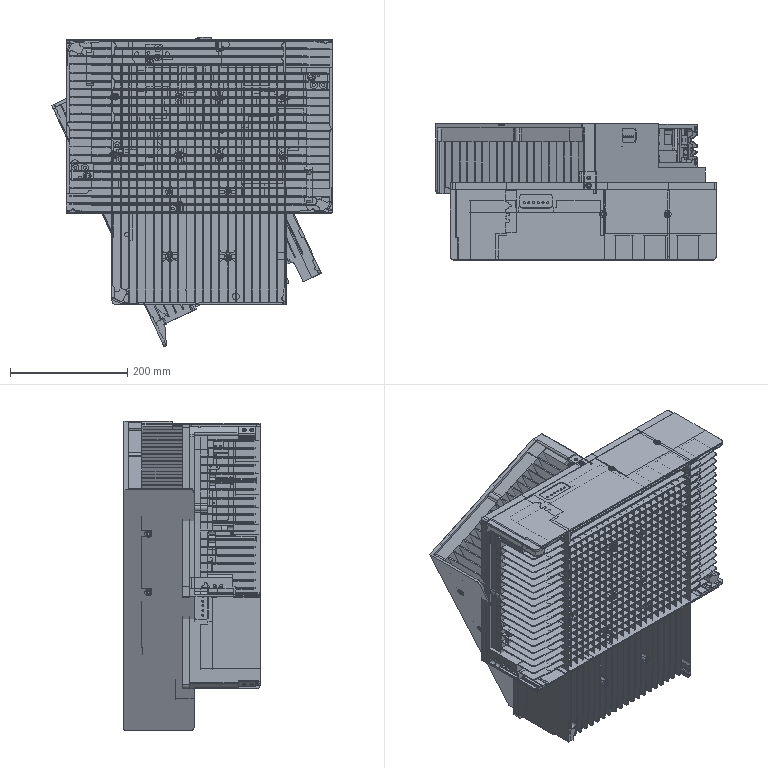NC program | NX | posted with a generic post
Whole program:
N10 G17 G21 G94 G90
(HOLE_MILLING_4 , TOOL : D4_J)
N12 T05 M6
N14 G53
N16 G17 G0 G90 X9.346 Y7. S2500 M3
N18 G43 Z20. H5
N20 Z0.1
N22 G94 G3 X9.846 Y6.5 R0.5 F1000.
N24 X10.346 Y7. R0.5
N26 X10.346 Y7. Z0.05 I-1. J0.
N28 X10.346 Y7. Z0. I-1. J0.
N30 X10.346 Y7. Z-0.05 I-1. J0.
N32 X10.346 Y7. Z-0.1 I-1. J0.
N34 X10.346 Y7. Z-0.15 I-1. J0.
N36 X10.346 Y7. Z-0.2 I-1. J0.
N38 X10.346 Y7. Z-0.25 I-1. J0.
N40 X10.346 Y7. Z-0.3 I-1. J0.
N42 X10.346 Y7. Z-0.35 I-1. J0.
N44 X10.346 Y7. Z-0.4 I-1. J0.
N46 X10.346 Y7. Z-0.45 I-1. J0.
N48 X10.346 Y7. Z-0.5 I-1. J0.
N50 X10.346 Y7. Z-0.55 I-1. J0.
N52 X10.346 Y7. Z-0.6 I-1. J0.
N54 X10.346 Y7. Z-0.65 I-1. J0.
N56 X10.346 Y7. Z-0.7 I-1. J0.
N58 X10.346 Y7. Z-0.75 I-1. J0.
N60 X10.346 Y7. Z-0.8 I-1. J0.
N62 X10.346 Y7. Z-0.85 I-1. J0.
N64 X10.346 Y7. Z-0.9 I-1. J0.
N66 X10.346 Y7. Z-0.95 I-1. J0.
N68 X10.346 Y7. Z-1. I-1. J0.
N70 X10.346 Y7. Z-1.05 I-1. J0.
N72 X10.346 Y7. Z-1.1 I-1. J0.
N74 X10.346 Y7. Z-1.15 I-1. J0.
N76 X10.346 Y7. Z-1.2 I-1. J0.
N78 X10.346 Y7. Z-1.25 I-1. J0.
N80 X10.346 Y7. Z-1.3 I-1. J0.
N82 X10.346 Y7. Z-1.35 I-1. J0.
N84 X10.346 Y7. Z-1.4 I-1. J0.
N86 X10.346 Y7. Z-1.45 I-1. J0.
N88 X10.346 Y7. Z-1.5 I-1. J0.
N90 X10.346 Y7. Z-1.55 I-1. J0.
N92 X10.346 Y7. Z-1.6 I-1. J0.
N94 X10.346 Y7. Z-1.65 I-1. J0.
N96 X10.346 Y7. Z-1.7 I-1. J0.
N98 X10.346 Y7. Z-1.75 I-1. J0.
N100 X10.346 Y7. Z-1.8 I-1. J0.
N102 X10.346 Y7. Z-1.85 I-1. J0.
N104 X10.346 Y7. Z-1.9 I-1. J0.
N106 X10.346 Y7. Z-1.95 I-1. J0.
N108 X10.346 Y7. Z-2. I-1. J0.
N110 X10.346 Y7. Z-2.05 I-1. J0.
N112 X10.346 Y7. Z-2.1 I-1. J0.
N114 X10.346 Y7. Z-2.15 I-1. J0.
N116 X10.346 Y7. Z-2.2 I-1. J0.
N118 X10.346 Y7. Z-2.25 I-1. J0.
N120 X10.346 Y7. Z-2.3 I-1. J0.
N122 X10.346 Y7. Z-2.35 I-1. J0.
N124 X10.346 Y7. Z-2.4 I-1. J0.
N126 X10.346 Y7. Z-2.45 I-1. J0.
N128 X10.346 Y7. Z-2.5 I-1. J0.
N130 X10.346 Y7. Z-2.55 I-1. J0.
N132 X10.346 Y7. Z-2.6 I-1. J0.
N134 X10.346 Y7. Z-2.65 I-1. J0.
N136 X10.346 Y7. Z-2.7 I-1. J0.
N138 X10.346 Y7. Z-2.75 I-1. J0.
N140 X10.346 Y7. Z-2.8 I-1. J0.
N142 X10.346 Y7. Z-2.85 I-1. J0.
N144 X10.346 Y7. Z-2.9 I-1. J0.
N146 X10.346 Y7. Z-2.95 I-1. J0.
N148 X10.346 Y7. Z-3. I-1. J0.
N150 X10.346 Y7. Z-3.05 I-1. J0.
N152 X10.346 Y7. Z-3.1 I-1. J0.
N154 X10.346 Y7. Z-3.15 I-1. J0.
N156 X10.346 Y7. Z-3.2 I-1. J0.
N158 X10.346 Y7. Z-3.25 I-1. J0.
N160 X10.346 Y7. Z-3.3 I-1. J0.
N162 X10.346 Y7. Z-3.35 I-1. J0.
N164 X10.346 Y7. Z-3.4 I-1. J0.
N166 X10.346 Y7. Z-3.45 I-1. J0.
N168 X10.346 Y7. Z-3.5 I-1. J0.
N170 X10.346 Y7. Z-3.55 I-1. J0.
N172 X10.346 Y7. Z-3.6 I-1. J0.
N174 X10.346 Y7. Z-3.65 I-1. J0.
N176 X10.346 Y7. Z-3.7 I-1. J0.
N178 X10.346 Y7. Z-3.75 I-1. J0.
N180 X10.346 Y7. Z-3.8 I-1. J0.
N182 X10.346 Y7. Z-3.85 I-1. J0.
N184 X10.346 Y7. Z-3.9 I-1. J0.
N186 X10.346 Y7. Z-3.95 I-1. J0.
N188 X10.346 Y7. Z-4. I-1. J0.
N190 X10.346 Y7. Z-4.05 I-1. J0.
N192 X10.346 Y7. Z-4.1 I-1. J0.
N194 X10.346 Y7. Z-4.15 I-1. J0.
N196 X10.346 Y7. Z-4.2 I-1. J0.
N198 X10.346 Y7. Z-4.25 I-1. J0.
N200 X10.346 Y7. Z-4.3 I-1. J0.
N202 X10.346 Y7. Z-4.35 I-1. J0.
N204 X10.346 Y7. Z-4.4 I-1. J0.
N206 X10.346 Y7. Z-4.45 I-1. J0.
N208 X10.346 Y7. Z-4.5 I-1. J0.
N210 X10.346 Y7. Z-4.55 I-1. J0.
N212 X10.346 Y7. Z-4.6 I-1. J0.
N214 X10.346 Y7. Z-4.65 I-1. J0.
N216 X10.346 Y7. Z-4.7 I-1. J0.
N218 X10.346 Y7. Z-4.75 I-1. J0.
N220 X10.346 Y7. Z-4.8 I-1. J0.
N222 X10.346 Y7. Z-4.85 I-1. J0.
N224 X10.346 Y7. Z-4.9 I-1. J0.
N226 X10.346 Y7. Z-4.95 I-1. J0.
N228 X10.346 Y7. Z-5. I-1. J0.
N230 X10.346 Y7. Z-5.05 I-1. J0.
N232 X10.346 Y7. Z-5.1 I-1. J0.
N234 X10.346 Y7. Z-5.15 I-1. J0.
N236 X10.346 Y7. Z-5.2 I-1. J0.
N238 X10.346 Y7. Z-5.25 I-1. J0.
N240 X10.346 Y7. Z-5.3 I-1. J0.
N242 X10.346 Y7. Z-5.35 I-1. J0.
N244 X10.346 Y7. Z-5.4 I-1. J0.
N246 X10.346 Y7. Z-5.45 I-1. J0.
N248 X10.346 Y7. Z-5.5 I-1. J0.
N250 X10.346 Y7. Z-5.55 I-1. J0.
N252 X10.346 Y7. Z-5.6 I-1. J0.
N254 X10.346 Y7. Z-5.65 I-1. J0.
N256 X10.346 Y7. Z-5.7 I-1. J0.
N258 X10.346 Y7. Z-5.75 I-1. J0.
N260 X10.346 Y7. Z-5.8 I-1. J0.
N262 X10.346 Y7. Z-5.85 I-1. J0.
N264 X10.346 Y7. Z-5.9 I-1. J0.
N266 X10.346 Y7. Z-5.95 I-1. J0.
N268 X10.346 Y7. Z-6. I-1. J0.
N270 X10.346 Y7. Z-6.05 I-1. J0.
N272 X10.346 Y7. Z-6.1 I-1. J0.
N274 X10.346 Y7. Z-6.15 I-1. J0.
N276 X10.346 Y7. Z-6.2 I-1. J0.
N278 X10.346 Y7. Z-6.25 I-1. J0.
N280 X10.346 Y7. Z-6.3 I-1. J0.
N282 X10.346 Y7. Z-6.35 I-1. J0.
N284 X10.346 Y7. Z-6.4 I-1. J0.
N286 X10.346 Y7. Z-6.45 I-1. J0.
N288 X10.346 Y7. Z-6.5 I-1. J0.
N290 X10.346 Y7. Z-6.55 I-1. J0.
N292 X10.346 Y7. Z-6.6 I-1. J0.
N294 X10.346 Y7. Z-6.65 I-1. J0.
N296 X10.346 Y7. Z-6.7 I-1. J0.
N298 X10.346 Y7. Z-6.75 I-1. J0.
N300 X10.346 Y7. Z-6.8 I-1. J0.
N302 X10.346 Y7. Z-6.85 I-1. J0.
N304 X10.346 Y7. Z-6.9 I-1. J0.
N306 X10.346 Y7. Z-6.95 I-1. J0.
N308 X10.346 Y7. Z-7. I-1. J0.
N310 X10.346 Y7. Z-7.05 I-1. J0.
N312 X10.346 Y7. Z-7.1 I-1. J0.
N314 X10.346 Y7. Z-7.15 I-1. J0.
N316 X10.346 Y7. Z-7.2 I-1. J0.
N318 X10.346 Y7. Z-7.25 I-1. J0.
N320 X10.346 Y7. Z-7.3 I-1. J0.
N322 X10.346 Y7. Z-7.35 I-1. J0.
N324 X10.346 Y7. Z-7.4 I-1. J0.
N326 X10.346 Y7. Z-7.45 I-1. J0.
N328 X10.346 Y7. Z-7.5 I-1. J0.
N330 X10.346 Y7. Z-7.55 I-1. J0.
N332 X10.346 Y7. Z-7.6 I-1. J0.
N334 X10.346 Y7. Z-7.65 I-1. J0.
N336 X10.346 Y7. Z-7.7 I-1. J0.
N338 X10.346 Y7. Z-7.75 I-1. J0.
N340 X10.346 Y7. Z-7.8 I-1. J0.
N342 X10.346 Y7. Z-7.85 I-1. J0.
N344 X10.346 Y7. Z-7.9 I-1. J0.
N346 X10.346 Y7. Z-7.95 I-1. J0.
N348 X10.346 Y7. Z-8. I-1. J0.
N350 X10.346 Y7. Z-8.05 I-1. J0.
N352 X10.346 Y7. Z-8.1 I-1. J0.
N354 X10.346 Y7. Z-8.15 I-1. J0.
N356 X10.346 Y7. Z-8.2 I-1. J0.
N358 X10.346 Y7. Z-8.25 I-1. J0.
N360 X10.346 Y7. Z-8.3 I-1. J0.
N362 X10.346 Y7. Z-8.35 I-1. J0.
N364 X10.346 Y7. Z-8.4 I-1. J0.
N366 X10.346 Y7. Z-8.45 I-1. J0.
N368 X10.346 Y7. Z-8.5 I-1. J0.
N370 X10.346 Y7. Z-8.55 I-1. J0.
N372 X10.346 Y7. Z-8.6 I-1. J0.
N374 X10.346 Y7. Z-8.65 I-1. J0.
N376 X10.346 Y7. Z-8.7 I-1. J0.
N378 X10.346 Y7. Z-8.75 I-1. J0.
N380 X10.346 Y7. Z-8.8 I-1. J0.
N382 X10.346 Y7. Z-8.85 I-1. J0.
N384 X10.346 Y7. Z-8.9 I-1. J0.
N386 X10.346 Y7. Z-8.95 I-1. J0.
N388 X10.346 Y7. Z-9. I-1. J0.
N390 X10.346 Y7. Z-9.05 I-1. J0.
N392 X10.346 Y7. Z-9.1 I-1. J0.
N394 X10.346 Y7. Z-9.15 I-1. J0.
N396 X10.346 Y7. Z-9.2 I-1. J0.
N398 X10.346 Y7. Z-9.25 I-1. J0.
N400 X10.346 Y7. Z-9.3 I-1. J0.
N402 X10.346 Y7. Z-9.35 I-1. J0.
N404 X10.346 Y7. Z-9.4 I-1. J0.
N406 X10.346 Y7. Z-9.45 I-1. J0.
N408 X10.346 Y7. Z-9.5 I-1. J0.
N410 X10.346 Y7. Z-9.55 I-1. J0.
N412 X10.346 Y7. Z-9.6 I-1. J0.
N414 X10.346 Y7. Z-9.65 I-1. J0.
N416 X10.346 Y7. Z-9.7 I-1. J0.
N418 X10.346 Y7. Z-9.75 I-1. J0.
N420 X10.346 Y7. Z-9.8 I-1. J0.
N422 X10.346 Y7. Z-9.85 I-1. J0.
N424 X10.346 Y7. Z-9.9 I-1. J0.
N426 X10.346 Y7. Z-9.95 I-1. J0.
N428 X10.346 Y7. Z-10. I-1. J0.
N430 X10.346 Y7. Z-10.05 I-1. J0.
N432 X10.346 Y7. Z-10.1 I-1. J0.
N434 X10.346 Y7. Z-10.15 I-1. J0.
N436 X10.346 Y7. Z-10.2 I-1. J0.
N438 X10.346 Y7. Z-10.25 I-1. J0.
N440 X10.346 Y7. Z-10.3 I-1. J0.
N442 X10.346 Y7. Z-10.35 I-1. J0.
N444 X10.346 Y7. Z-10.4 I-1. J0.
N446 X10.346 Y7. Z-10.45 I-1. J0.
N448 X10.346 Y7. Z-10.5 I-1. J0.
N450 X10.346 Y7. Z-10.55 I-1. J0.
N452 X10.346 Y7. Z-10.6 I-1. J0.
N454 X10.346 Y7. Z-10.65 I-1. J0.
N456 X10.346 Y7. Z-10.7 I-1. J0.
N458 X10.346 Y7. Z-10.75 I-1. J0.
N460 X10.346 Y7. Z-10.8 I-1. J0.
N462 X10.346 Y7. Z-10.85 I-1. J0.
N464 X10.346 Y7. Z-10.9 I-1. J0.
N466 X10.346 Y7. Z-10.95 I-1. J0.
N468 X10.346 Y7. Z-11. I-1. J0.
N470 X10.346 Y7. Z-11.05 I-1. J0.
N472 X10.346 Y7. Z-11.1 I-1. J0.
N474 X10.346 Y7. Z-11.15 I-1. J0.
N476 X10.346 Y7. Z-11.2 I-1. J0.
N478 X10.346 Y7. Z-11.25 I-1. J0.
N480 X10.346 Y7. Z-11.3 I-1. J0.
N482 X10.346 Y7. Z-11.35 I-1. J0.
N484 X10.346 Y7. Z-11.4 I-1. J0.
N486 X10.346 Y7. Z-11.45 I-1. J0.
N488 X10.346 Y7. Z-11.5 I-1. J0.
N490 X10.346 Y7. Z-11.55 I-1. J0.
N492 X10.346 Y7. Z-11.6 I-1. J0.
N494 X10.346 Y7. Z-11.65 I-1. J0.
N496 X10.346 Y7. Z-11.7 I-1. J0.
N498 X10.346 Y7. Z-11.75 I-1. J0.
N500 X10.346 Y7. Z-11.8 I-1. J0.
N502 X10.346 Y7. Z-11.85 I-1. J0.
N504 X10.346 Y7. Z-11.9 I-1. J0.
N506 X10.346 Y7. Z-11.95 I-1. J0.
N508 X10.346 Y7. Z-12. I-1. J0.
N510 X10.346 Y7. Z-12.05 I-1. J0.
N512 X10.346 Y7. Z-12.1 I-1. J0.
N514 X10.346 Y7. Z-12.15 I-1. J0.
N516 X10.346 Y7. Z-12.2 I-1. J0.
N518 X10.346 Y7. Z-12.25 I-1. J0.
N520 X10.346 Y7. Z-12.3 I-1. J0.
N522 X10.346 Y7. Z-12.35 I-1. J0.
N524 X10.346 Y7. Z-12.4 I-1. J0.
N526 X10.346 Y7. Z-12.45 I-1. J0.
N528 X10.346 Y7. Z-12.5 I-1. J0.
N530 X10.346 Y7. Z-12.55 I-1. J0.
N532 X10.346 Y7. Z-12.6 I-1. J0.
N534 X10.346 Y7. Z-12.65 I-1. J0.
N536 X10.346 Y7. Z-12.7 I-1. J0.
N538 X10.346 Y7. Z-12.75 I-1. J0.
N540 X10.346 Y7. Z-12.8 I-1. J0.
N542 X10.346 Y7. Z-12.85 I-1. J0.
N544 X10.346 Y7. Z-12.9 I-1. J0.
N546 X10.346 Y7. Z-12.95 I-1. J0.
N548 X10.346 Y7. Z-13. I-1. J0.
N550 X10.346 Y7. Z-13.05 I-1. J0.
N552 X10.346 Y7. Z-13.1 I-1. J0.
N554 X10.346 Y7. Z-13.15 I-1. J0.
N556 X10.346 Y7. Z-13.2 I-1. J0.
N558 X10.346 Y7. Z-13.25 I-1. J0.
N560 X10.346 Y7. Z-13.3 I-1. J0.
N562 X10.346 Y7. Z-13.35 I-1. J0.
N564 X10.346 Y7. Z-13.4 I-1. J0.
N566 X10.346 Y7. Z-13.45 I-1. J0.
N568 X10.346 Y7. Z-13.5 I-1. J0.
N570 X10.346 Y7. Z-13.55 I-1. J0.
N572 X10.346 Y7. Z-13.6 I-1. J0.
N574 X10.346 Y7. Z-13.65 I-1. J0.
N576 X10.346 Y7. Z-13.7 I-1. J0.
N578 X10.346 Y7. Z-13.75 I-1. J0.
N580 X10.346 Y7. Z-13.8 I-1. J0.
N582 X10.346 Y7. Z-13.85 I-1. J0.
N584 X10.346 Y7. Z-13.9 I-1. J0.
N586 X10.346 Y7. Z-13.95 I-1. J0.
N588 X10.346 Y7. Z-14. I-1. J0.
N590 X10.346 Y7. Z-14.05 I-1. J0.
N592 X10.346 Y7. Z-14.1 I-1. J0.
N594 X10.346 Y7. Z-14.15 I-1. J0.
N596 X10.346 Y7. Z-14.2 I-1. J0.
N598 X10.346 Y7. Z-14.25 I-1. J0.
N600 X10.346 Y7. Z-14.3 I-1. J0.
N602 X10.346 Y7. Z-14.35 I-1. J0.
N604 X10.346 Y7. Z-14.4 I-1. J0.
N606 X10.346 Y7. Z-14.45 I-1. J0.
N608 X10.346 Y7. Z-14.5 I-1. J0.
N610 X10.346 Y7. Z-14.55 I-1. J0.
N612 X10.346 Y7. Z-14.6 I-1. J0.
N614 X10.346 Y7. Z-14.65 I-1. J0.
N616 X10.346 Y7. Z-14.7 I-1. J0.
N618 X10.346 Y7. Z-14.75 I-1. J0.
N620 X10.346 Y7. Z-14.8 I-1. J0.
N622 X10.346 Y7. Z-14.85 I-1. J0.
N624 X10.346 Y7. Z-14.9 I-1. J0.
N626 X10.346 Y7. Z-14.95 I-1. J0.
N628 X10.346 Y7. Z-15. I-1. J0.
N630 X9.346 Y8. R1.
N632 X10.346 Y7. R-1.
N634 X9.846 Y7.5 R0.5
N636 X9.346 Y7. R0.5
N638 G0 Z20.
N640 M5
N642 M2